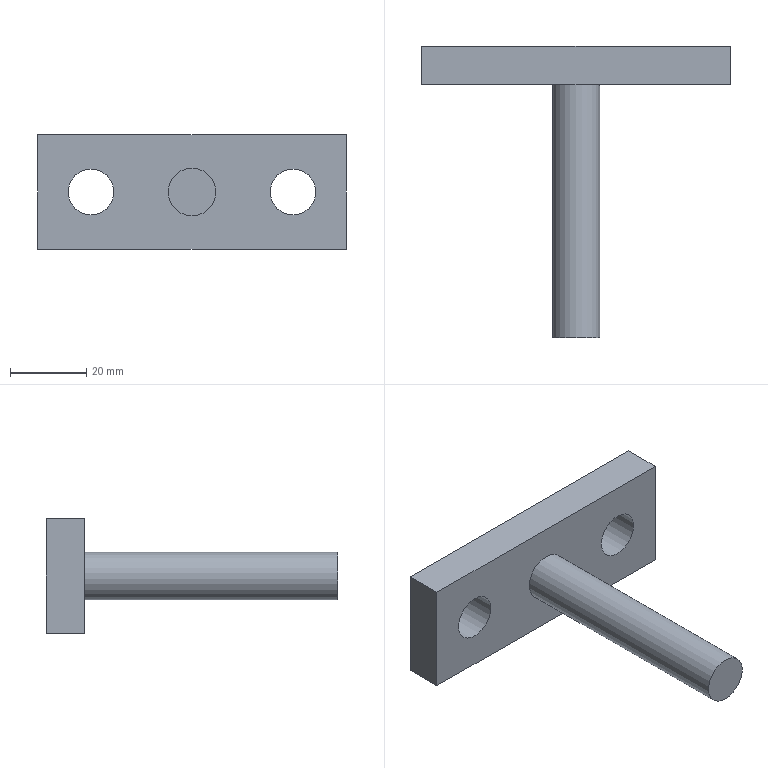Part | STEP file | Tube necking machine_id10_x_t | 1 solid | 10 faces | box 81 x 76.5 x 30 mm | volume 30169 mm3 | plane 7 | cylinder 3 | commonest cylinder face diameters 12 x2 12.477 x1
STEP:
#1=CARTESIAN_POINT('',(0.,0.,0.));
#2=DIRECTION('',(0.,0.,1.));
#3=DIRECTION('',(1.,0.,0.));
#4=AXIS2_PLACEMENT_3D('',#1,#2,#3);
#5=CARTESIAN_POINT('',(26.5,-259.,195.));
#6=VERTEX_POINT('',#5);
#7=CARTESIAN_POINT('',(26.5,-259.,183.));
#8=VERTEX_POINT('',#7);
#9=CARTESIAN_POINT('',(26.5,-259.,189.));
#10=DIRECTION('',(0.,1.,0.));
#11=DIRECTION('',(0.,0.,-1.));
#12=AXIS2_PLACEMENT_3D('',#9,#10,#11);
#13=CIRCLE('',#12,6.);
#14=CARTESIAN_POINT('',(26.5,-807.,189.));
#15=DIRECTION('',(0.,1.,0.));
#16=DIRECTION('',(0.,0.,1.));
#17=AXIS2_PLACEMENT_3D('',#14,#15,#16);
#18=CYLINDRICAL_SURFACE('',#17,6.);
#19=CARTESIAN_POINT('',(-3.142,548.));
#20=DIRECTION('',(1.,0.));
#21=VECTOR('',#20,1.);
#22=LINE('',#19,#21);
#23=(GEOMETRIC_REPRESENTATION_CONTEXT(2)PARAMETRIC_REPRESENTATION_CONTEXT()REPRESENTATION_CONTEXT('',''));
#24=DEFINITIONAL_REPRESENTATION('',(#22),#23);
#25=PCURVE('',#18,#24);
#26=CARTESIAN_POINT('',(0.,-259.,0.));
#27=DIRECTION('',(0.,-1.,0.));
#28=DIRECTION('',(0.,0.,-1.));
#29=AXIS2_PLACEMENT_3D('',#26,#27,#28);
#30=PLANE('',#29);
#31=CARTESIAN_POINT('',(-183.,26.5));
#32=CARTESIAN_POINT('',(-183.,16.108));
#33=CARTESIAN_POINT('',(-192.,21.304));
#34=CARTESIAN_POINT('',(-201.,26.5));
#35=CARTESIAN_POINT('',(-192.,31.696));
#36=CARTESIAN_POINT('',(-183.,36.892));
#37=CARTESIAN_POINT('',(-183.,26.5));
#38=(BOUNDED_CURVE()B_SPLINE_CURVE(2,(#31,#32,#33,#34,#35,#36,#37),.UNSPECIFIED.,.T.,.F.)B_SPLINE_CURVE_WITH_KNOTS((1,2,2,2,2,1),(-2.094,0.,2.094,4.189,6.283,8.378),.UNSPECIFIED.)CURVE()GEOMETRIC_REPRESENTATION_ITEM()RATIONAL_B_SPLINE_CURVE((1.,0.5,1.,0.5,1.,0.5,1.))REPRESENTATION_ITEM(''));
#39=(GEOMETRIC_REPRESENTATION_CONTEXT(2)PARAMETRIC_REPRESENTATION_CONTEXT()REPRESENTATION_CONTEXT('',''));
#40=DEFINITIONAL_REPRESENTATION('',(#38),#39);
#41=PCURVE('',#30,#40);
#42=SURFACE_CURVE('',#13,(#25,#41),.PCURVE_S1.);
#43=EDGE_CURVE('',#6,#8,#42,.T.);
#44=ORIENTED_EDGE('',*,*,#43,.F.);
#45=CARTESIAN_POINT('',(26.5,-269.,195.));
#46=VERTEX_POINT('',#45);
#47=CARTESIAN_POINT('',(26.5,-269.,195.));
#48=CARTESIAN_POINT('',(26.5,-259.,195.));
#49=B_SPLINE_CURVE_WITH_KNOTS('',1,(#47,#48),.UNSPECIFIED.,.F.,.F.,(2,2),(538.,548.),.PIECEWISE_BEZIER_KNOTS.);
#50=CARTESIAN_POINT('',(0.,0.));
#51=DIRECTION('',(0.,1.));
#52=VECTOR('',#51,1.);
#53=LINE('',#50,#52);
#54=(GEOMETRIC_REPRESENTATION_CONTEXT(2)PARAMETRIC_REPRESENTATION_CONTEXT()REPRESENTATION_CONTEXT('',''));
#55=DEFINITIONAL_REPRESENTATION('',(#53),#54);
#56=PCURVE('',#18,#55);
#57=CARTESIAN_POINT('',(6.283,0.));
#58=DIRECTION('',(0.,1.));
#59=VECTOR('',#58,1.);
#60=LINE('',#57,#59);
#61=(GEOMETRIC_REPRESENTATION_CONTEXT(2)PARAMETRIC_REPRESENTATION_CONTEXT()REPRESENTATION_CONTEXT('',''));
#62=DEFINITIONAL_REPRESENTATION('',(#60),#61);
#63=PCURVE('',#18,#62);
#64=SEAM_CURVE('',#49,(#56,#63),.PCURVE_S1.);
#65=EDGE_CURVE('',#46,#6,#64,.T.);
#66=ORIENTED_EDGE('',*,*,#65,.F.);
#67=CARTESIAN_POINT('',(26.5,-269.,189.));
#68=DIRECTION('',(0.,-1.,0.));
#69=DIRECTION('',(0.,0.,1.));
#70=AXIS2_PLACEMENT_3D('',#67,#68,#69);
#71=CIRCLE('',#70,6.);
#72=CARTESIAN_POINT('',(6.283,538.));
#73=DIRECTION('',(-1.,0.));
#74=VECTOR('',#73,1.);
#75=LINE('',#72,#74);
#76=(GEOMETRIC_REPRESENTATION_CONTEXT(2)PARAMETRIC_REPRESENTATION_CONTEXT()REPRESENTATION_CONTEXT('',''));
#77=DEFINITIONAL_REPRESENTATION('',(#75),#76);
#78=PCURVE('',#18,#77);
#79=CARTESIAN_POINT('',(0.,-269.,0.));
#80=DIRECTION('',(0.,1.,0.));
#81=DIRECTION('',(0.,0.,1.));
#82=AXIS2_PLACEMENT_3D('',#79,#80,#81);
#83=PLANE('',#82);
#84=CARTESIAN_POINT('',(195.,26.5));
#85=CARTESIAN_POINT('',(195.,16.108));
#86=CARTESIAN_POINT('',(186.,21.304));
#87=CARTESIAN_POINT('',(177.,26.5));
#88=CARTESIAN_POINT('',(186.,31.696));
#89=CARTESIAN_POINT('',(195.,36.892));
#90=CARTESIAN_POINT('',(195.,26.5));
#91=(BOUNDED_CURVE()B_SPLINE_CURVE(2,(#84,#85,#86,#87,#88,#89,#90),.UNSPECIFIED.,.T.,.F.)B_SPLINE_CURVE_WITH_KNOTS((1,2,2,2,2,1),(-2.094,0.,2.094,4.189,6.283,8.378),.UNSPECIFIED.)CURVE()GEOMETRIC_REPRESENTATION_ITEM()RATIONAL_B_SPLINE_CURVE((1.,0.5,1.,0.5,1.,0.5,1.))REPRESENTATION_ITEM(''));
#92=(GEOMETRIC_REPRESENTATION_CONTEXT(2)PARAMETRIC_REPRESENTATION_CONTEXT()REPRESENTATION_CONTEXT('',''));
#93=DEFINITIONAL_REPRESENTATION('',(#91),#92);
#94=PCURVE('',#83,#93);
#95=SURFACE_CURVE('',#71,(#78,#94),.PCURVE_S1.);
#96=EDGE_CURVE('',#46,#46,#95,.T.);
#97=ORIENTED_EDGE('',*,*,#96,.F.);
#98=ORIENTED_EDGE('',*,*,#65,.T.);
#99=CARTESIAN_POINT('',(26.5,-259.,189.));
#100=DIRECTION('',(0.,1.,0.));
#101=DIRECTION('',(0.,0.,-1.));
#102=AXIS2_PLACEMENT_3D('',#99,#100,#101);
#103=CIRCLE('',#102,6.);
#104=CARTESIAN_POINT('',(3.142,548.));
#105=DIRECTION('',(1.,0.));
#106=VECTOR('',#105,1.);
#107=LINE('',#104,#106);
#108=(GEOMETRIC_REPRESENTATION_CONTEXT(2)PARAMETRIC_REPRESENTATION_CONTEXT()REPRESENTATION_CONTEXT('',''));
#109=DEFINITIONAL_REPRESENTATION('',(#107),#108);
#110=PCURVE('',#18,#109);
#111=CARTESIAN_POINT('',(-183.,26.5));
#112=CARTESIAN_POINT('',(-183.,16.108));
#113=CARTESIAN_POINT('',(-192.,21.304));
#114=CARTESIAN_POINT('',(-201.,26.5));
#115=CARTESIAN_POINT('',(-192.,31.696));
#116=CARTESIAN_POINT('',(-183.,36.892));
#117=CARTESIAN_POINT('',(-183.,26.5));
#118=(BOUNDED_CURVE()B_SPLINE_CURVE(2,(#111,#112,#113,#114,#115,#116,#117),.UNSPECIFIED.,.T.,.F.)B_SPLINE_CURVE_WITH_KNOTS((1,2,2,2,2,1),(-2.094,0.,2.094,4.189,6.283,8.378),.UNSPECIFIED.)CURVE()GEOMETRIC_REPRESENTATION_ITEM()RATIONAL_B_SPLINE_CURVE((1.,0.5,1.,0.5,1.,0.5,1.))REPRESENTATION_ITEM(''));
#119=(GEOMETRIC_REPRESENTATION_CONTEXT(2)PARAMETRIC_REPRESENTATION_CONTEXT()REPRESENTATION_CONTEXT('',''));
#120=DEFINITIONAL_REPRESENTATION('',(#118),#119);
#121=PCURVE('',#30,#120);
#122=SURFACE_CURVE('',#103,(#110,#121),.PCURVE_S1.);
#123=EDGE_CURVE('',#8,#6,#122,.T.);
#124=ORIENTED_EDGE('',*,*,#123,.F.);
#125=EDGE_LOOP('',(#44,#66,#97,#98,#124));
#126=FACE_BOUND('',#125,.F.);
#127=ADVANCED_FACE('',(#126),#18,.F.);
#128=CARTESIAN_POINT('',(0.,-335.5,182.761));
#129=VERTEX_POINT('',#128);
#130=CARTESIAN_POINT('',(0.,-335.5,189.));
#131=DIRECTION('',(0.,1.,0.));
#132=DIRECTION('',(0.,0.,-1.));
#133=AXIS2_PLACEMENT_3D('',#130,#131,#132);
#134=CIRCLE('',#133,6.239);
#135=CARTESIAN_POINT('',(-26.5,-335.5,189.));
#136=DIRECTION('',(0.,-1.,0.));
#137=DIRECTION('',(0.,0.,-1.));
#138=AXIS2_PLACEMENT_3D('',#135,#136,#137);
#139=PLANE('',#138);
#140=CARTESIAN_POINT('',(6.239,26.5));
#141=CARTESIAN_POINT('',(6.239,15.694));
#142=CARTESIAN_POINT('',(-3.119,21.097));
#143=CARTESIAN_POINT('',(-12.477,26.5));
#144=CARTESIAN_POINT('',(-3.119,31.903));
#145=CARTESIAN_POINT('',(6.239,37.306));
#146=CARTESIAN_POINT('',(6.239,26.5));
#147=(BOUNDED_CURVE()B_SPLINE_CURVE(2,(#140,#141,#142,#143,#144,#145,#146),.UNSPECIFIED.,.T.,.F.)B_SPLINE_CURVE_WITH_KNOTS((1,2,2,2,2,1),(-2.094,0.,2.094,4.189,6.283,8.378),.UNSPECIFIED.)CURVE()GEOMETRIC_REPRESENTATION_ITEM()RATIONAL_B_SPLINE_CURVE((1.,0.5,1.,0.5,1.,0.5,1.))REPRESENTATION_ITEM(''));
#148=(GEOMETRIC_REPRESENTATION_CONTEXT(2)PARAMETRIC_REPRESENTATION_CONTEXT()REPRESENTATION_CONTEXT('',''));
#149=DEFINITIONAL_REPRESENTATION('',(#147),#148);
#150=PCURVE('',#139,#149);
#151=CARTESIAN_POINT('',(0.,-262.,189.));
#152=DIRECTION('',(0.,-1.,0.));
#153=DIRECTION('',(0.,0.,-1.));
#154=AXIS2_PLACEMENT_3D('',#151,#152,#153);
#155=CYLINDRICAL_SURFACE('',#154,6.239);
#156=CARTESIAN_POINT('',(6.283,73.5));
#157=DIRECTION('',(-1.,0.));
#158=VECTOR('',#157,1.);
#159=LINE('',#156,#158);
#160=(GEOMETRIC_REPRESENTATION_CONTEXT(2)PARAMETRIC_REPRESENTATION_CONTEXT()REPRESENTATION_CONTEXT('',''));
#161=DEFINITIONAL_REPRESENTATION('',(#159),#160);
#162=PCURVE('',#155,#161);
#163=SURFACE_CURVE('',#134,(#150,#162),.PCURVE_S1.);
#164=EDGE_CURVE('',#129,#129,#163,.T.);
#165=ORIENTED_EDGE('',*,*,#164,.F.);
#166=EDGE_LOOP('',(#165));
#167=FACE_BOUND('',#166,.T.);
#168=ADVANCED_FACE('',(#167),#139,.T.);
#169=ORIENTED_EDGE('',*,*,#164,.T.);
#170=CARTESIAN_POINT('',(0.,-269.,182.761));
#171=VERTEX_POINT('',#170);
#172=CARTESIAN_POINT('',(0.,-269.,182.761));
#173=CARTESIAN_POINT('',(0.,-335.5,182.761));
#174=B_SPLINE_CURVE_WITH_KNOTS('',1,(#172,#173),.UNSPECIFIED.,.F.,.F.,(2,2),(7.,73.5),.PIECEWISE_BEZIER_KNOTS.);
#175=CARTESIAN_POINT('',(0.,0.));
#176=DIRECTION('',(0.,1.));
#177=VECTOR('',#176,1.);
#178=LINE('',#175,#177);
#179=(GEOMETRIC_REPRESENTATION_CONTEXT(2)PARAMETRIC_REPRESENTATION_CONTEXT()REPRESENTATION_CONTEXT('',''));
#180=DEFINITIONAL_REPRESENTATION('',(#178),#179);
#181=PCURVE('',#155,#180);
#182=CARTESIAN_POINT('',(6.283,0.));
#183=DIRECTION('',(0.,1.));
#184=VECTOR('',#183,1.);
#185=LINE('',#182,#184);
#186=(GEOMETRIC_REPRESENTATION_CONTEXT(2)PARAMETRIC_REPRESENTATION_CONTEXT()REPRESENTATION_CONTEXT('',''));
#187=DEFINITIONAL_REPRESENTATION('',(#185),#186);
#188=PCURVE('',#155,#187);
#189=SEAM_CURVE('',#174,(#181,#188),.PCURVE_S1.);
#190=EDGE_CURVE('',#171,#129,#189,.T.);
#191=ORIENTED_EDGE('',*,*,#190,.F.);
#192=CARTESIAN_POINT('',(0.,-269.,195.239));
#193=VERTEX_POINT('',#192);
#194=CARTESIAN_POINT('',(0.,-269.,189.));
#195=DIRECTION('',(0.,1.,0.));
#196=DIRECTION('',(0.,0.,1.));
#197=AXIS2_PLACEMENT_3D('',#194,#195,#196);
#198=CIRCLE('',#197,6.239);
#199=CARTESIAN_POINT('',(3.142,7.));
#200=DIRECTION('',(-1.,0.));
#201=VECTOR('',#200,1.);
#202=LINE('',#199,#201);
#203=(GEOMETRIC_REPRESENTATION_CONTEXT(2)PARAMETRIC_REPRESENTATION_CONTEXT()REPRESENTATION_CONTEXT('',''));
#204=DEFINITIONAL_REPRESENTATION('',(#202),#203);
#205=PCURVE('',#155,#204);
#206=CARTESIAN_POINT('',(189.,0.));
#207=DIRECTION('',(1.,0.));
#208=AXIS2_PLACEMENT_2D('',#206,#207);
#209=CIRCLE('',#208,6.239);
#210=(GEOMETRIC_REPRESENTATION_CONTEXT(2)PARAMETRIC_REPRESENTATION_CONTEXT()REPRESENTATION_CONTEXT('',''));
#211=DEFINITIONAL_REPRESENTATION('',(#209),#210);
#212=PCURVE('',#83,#211);
#213=SURFACE_CURVE('',#198,(#205,#212),.PCURVE_S1.);
#214=EDGE_CURVE('',#193,#171,#213,.T.);
#215=ORIENTED_EDGE('',*,*,#214,.F.);
#216=CARTESIAN_POINT('',(0.,-269.,189.));
#217=DIRECTION('',(0.,1.,0.));
#218=DIRECTION('',(0.,0.,1.));
#219=AXIS2_PLACEMENT_3D('',#216,#217,#218);
#220=CIRCLE('',#219,6.239);
#221=CARTESIAN_POINT('',(9.425,7.));
#222=DIRECTION('',(-1.,0.));
#223=VECTOR('',#222,1.);
#224=LINE('',#221,#223);
#225=(GEOMETRIC_REPRESENTATION_CONTEXT(2)PARAMETRIC_REPRESENTATION_CONTEXT()REPRESENTATION_CONTEXT('',''));
#226=DEFINITIONAL_REPRESENTATION('',(#224),#225);
#227=PCURVE('',#155,#226);
#228=CARTESIAN_POINT('',(189.,0.));
#229=DIRECTION('',(1.,0.));
#230=AXIS2_PLACEMENT_2D('',#228,#229);
#231=CIRCLE('',#230,6.239);
#232=(GEOMETRIC_REPRESENTATION_CONTEXT(2)PARAMETRIC_REPRESENTATION_CONTEXT()REPRESENTATION_CONTEXT('',''));
#233=DEFINITIONAL_REPRESENTATION('',(#231),#232);
#234=PCURVE('',#83,#233);
#235=SURFACE_CURVE('',#220,(#227,#234),.PCURVE_S1.);
#236=EDGE_CURVE('',#171,#193,#235,.T.);
#237=ORIENTED_EDGE('',*,*,#236,.F.);
#238=ORIENTED_EDGE('',*,*,#190,.T.);
#239=EDGE_LOOP('',(#169,#191,#215,#237,#238));
#240=FACE_BOUND('',#239,.T.);
#241=ADVANCED_FACE('',(#240),#155,.T.);
#242=CARTESIAN_POINT('',(-40.5,-259.,204.));
#243=VERTEX_POINT('',#242);
#244=CARTESIAN_POINT('',(-40.5,-269.,204.));
#245=VERTEX_POINT('',#244);
#246=CARTESIAN_POINT('',(-40.5,-125.5,204.));
#247=DIRECTION('',(0.,-1.,0.));
#248=VECTOR('',#247,1.);
#249=LINE('',#246,#248);
#250=CARTESIAN_POINT('',(-40.5,-125.5,171.));
#251=DIRECTION('',(1.,0.,0.));
#252=DIRECTION('',(0.,0.,-1.));
#253=AXIS2_PLACEMENT_3D('',#250,#251,#252);
#254=PLANE('',#253);
#255=CARTESIAN_POINT('',(-33.,0.));
#256=DIRECTION('',(0.,-1.));
#257=VECTOR('',#256,1.);
#258=LINE('',#255,#257);
#259=(GEOMETRIC_REPRESENTATION_CONTEXT(2)PARAMETRIC_REPRESENTATION_CONTEXT()REPRESENTATION_CONTEXT('',''));
#260=DEFINITIONAL_REPRESENTATION('',(#258),#259);
#261=PCURVE('',#254,#260);
#262=CARTESIAN_POINT('',(-41.5,-125.5,204.));
#263=DIRECTION('',(0.,0.,-1.));
#264=DIRECTION('',(-1.,0.,0.));
#265=AXIS2_PLACEMENT_3D('',#262,#263,#264);
#266=PLANE('',#265);
#267=CARTESIAN_POINT('',(-1.,0.));
#268=DIRECTION('',(0.,-1.));
#269=VECTOR('',#268,1.);
#270=LINE('',#267,#269);
#271=(GEOMETRIC_REPRESENTATION_CONTEXT(2)PARAMETRIC_REPRESENTATION_CONTEXT()REPRESENTATION_CONTEXT('',''));
#272=DEFINITIONAL_REPRESENTATION('',(#270),#271);
#273=PCURVE('',#266,#272);
#274=SURFACE_CURVE('',#249,(#261,#273),.PCURVE_S1.);
#275=EDGE_CURVE('',#243,#245,#274,.T.);
#276=ORIENTED_EDGE('',*,*,#275,.F.);
#277=CARTESIAN_POINT('',(-40.5,-259.,174.));
#278=VERTEX_POINT('',#277);
#279=CARTESIAN_POINT('',(-40.5,-259.,171.));
#280=DIRECTION('',(0.,0.,-1.));
#281=VECTOR('',#280,1.);
#282=LINE('',#279,#281);
#283=CARTESIAN_POINT('',(0.,-133.5));
#284=DIRECTION('',(1.,0.));
#285=VECTOR('',#284,1.);
#286=LINE('',#283,#285);
#287=(GEOMETRIC_REPRESENTATION_CONTEXT(2)PARAMETRIC_REPRESENTATION_CONTEXT()REPRESENTATION_CONTEXT('',''));
#288=DEFINITIONAL_REPRESENTATION('',(#286),#287);
#289=PCURVE('',#254,#288);
#290=CARTESIAN_POINT('',(-171.,-40.5));
#291=DIRECTION('',(1.,0.));
#292=VECTOR('',#291,1.);
#293=LINE('',#290,#292);
#294=(GEOMETRIC_REPRESENTATION_CONTEXT(2)PARAMETRIC_REPRESENTATION_CONTEXT()REPRESENTATION_CONTEXT('',''));
#295=DEFINITIONAL_REPRESENTATION('',(#293),#294);
#296=PCURVE('',#30,#295);
#297=SURFACE_CURVE('',#282,(#289,#296),.PCURVE_S1.);
#298=EDGE_CURVE('',#243,#278,#297,.T.);
#299=ORIENTED_EDGE('',*,*,#298,.T.);
#300=CARTESIAN_POINT('',(-40.5,-269.,174.));
#301=VERTEX_POINT('',#300);
#302=CARTESIAN_POINT('',(-40.5,-125.5,174.));
#303=DIRECTION('',(0.,-1.,0.));
#304=VECTOR('',#303,1.);
#305=LINE('',#302,#304);
#306=CARTESIAN_POINT('',(-3.,0.));
#307=DIRECTION('',(0.,-1.));
#308=VECTOR('',#307,1.);
#309=LINE('',#306,#308);
#310=(GEOMETRIC_REPRESENTATION_CONTEXT(2)PARAMETRIC_REPRESENTATION_CONTEXT()REPRESENTATION_CONTEXT('',''));
#311=DEFINITIONAL_REPRESENTATION('',(#309),#310);
#312=PCURVE('',#254,#311);
#313=CARTESIAN_POINT('',(41.5,-125.5,174.));
#314=DIRECTION('',(0.,0.,1.));
#315=DIRECTION('',(1.,0.,0.));
#316=AXIS2_PLACEMENT_3D('',#313,#314,#315);
#317=PLANE('',#316);
#318=CARTESIAN_POINT('',(-82.,0.));
#319=DIRECTION('',(0.,-1.));
#320=VECTOR('',#319,1.);
#321=LINE('',#318,#320);
#322=(GEOMETRIC_REPRESENTATION_CONTEXT(2)PARAMETRIC_REPRESENTATION_CONTEXT()REPRESENTATION_CONTEXT('',''));
#323=DEFINITIONAL_REPRESENTATION('',(#321),#322);
#324=PCURVE('',#317,#323);
#325=SURFACE_CURVE('',#305,(#312,#324),.PCURVE_S1.);
#326=EDGE_CURVE('',#278,#301,#325,.T.);
#327=ORIENTED_EDGE('',*,*,#326,.T.);
#328=CARTESIAN_POINT('',(-40.5,-269.,171.));
#329=DIRECTION('',(0.,0.,1.));
#330=VECTOR('',#329,1.);
#331=LINE('',#328,#330);
#332=CARTESIAN_POINT('',(0.,-143.5));
#333=DIRECTION('',(-1.,0.));
#334=VECTOR('',#333,1.);
#335=LINE('',#332,#334);
#336=(GEOMETRIC_REPRESENTATION_CONTEXT(2)PARAMETRIC_REPRESENTATION_CONTEXT()REPRESENTATION_CONTEXT('',''));
#337=DEFINITIONAL_REPRESENTATION('',(#335),#336);
#338=PCURVE('',#254,#337);
#339=CARTESIAN_POINT('',(171.,-40.5));
#340=DIRECTION('',(1.,0.));
#341=VECTOR('',#340,1.);
#342=LINE('',#339,#341);
#343=(GEOMETRIC_REPRESENTATION_CONTEXT(2)PARAMETRIC_REPRESENTATION_CONTEXT()REPRESENTATION_CONTEXT('',''));
#344=DEFINITIONAL_REPRESENTATION('',(#342),#343);
#345=PCURVE('',#83,#344);
#346=SURFACE_CURVE('',#331,(#338,#345),.PCURVE_S1.);
#347=EDGE_CURVE('',#301,#245,#346,.T.);
#348=ORIENTED_EDGE('',*,*,#347,.T.);
#349=EDGE_LOOP('',(#276,#299,#327,#348));
#350=FACE_BOUND('',#349,.T.);
#351=ADVANCED_FACE('',(#350),#254,.F.);
#352=ORIENTED_EDGE('',*,*,#326,.F.);
#353=CARTESIAN_POINT('',(40.5,-259.,174.));
#354=VERTEX_POINT('',#353);
#355=CARTESIAN_POINT('',(41.5,-259.,174.));
#356=DIRECTION('',(1.,0.,0.));
#357=VECTOR('',#356,1.);
#358=LINE('',#355,#357);
#359=CARTESIAN_POINT('',(0.,-133.5));
#360=DIRECTION('',(1.,0.));
#361=VECTOR('',#360,1.);
#362=LINE('',#359,#361);
#363=(GEOMETRIC_REPRESENTATION_CONTEXT(2)PARAMETRIC_REPRESENTATION_CONTEXT()REPRESENTATION_CONTEXT('',''));
#364=DEFINITIONAL_REPRESENTATION('',(#362),#363);
#365=PCURVE('',#317,#364);
#366=CARTESIAN_POINT('',(-174.,41.5));
#367=DIRECTION('',(0.,1.));
#368=VECTOR('',#367,1.);
#369=LINE('',#366,#368);
#370=(GEOMETRIC_REPRESENTATION_CONTEXT(2)PARAMETRIC_REPRESENTATION_CONTEXT()REPRESENTATION_CONTEXT('',''));
#371=DEFINITIONAL_REPRESENTATION('',(#369),#370);
#372=PCURVE('',#30,#371);
#373=SURFACE_CURVE('',#358,(#365,#372),.PCURVE_S1.);
#374=EDGE_CURVE('',#278,#354,#373,.T.);
#375=ORIENTED_EDGE('',*,*,#374,.T.);
#376=CARTESIAN_POINT('',(40.5,-269.,174.));
#377=VERTEX_POINT('',#376);
#378=CARTESIAN_POINT('',(40.5,-125.5,174.));
#379=DIRECTION('',(0.,-1.,0.));
#380=VECTOR('',#379,1.);
#381=LINE('',#378,#380);
#382=CARTESIAN_POINT('',(-1.,0.));
#383=DIRECTION('',(0.,-1.));
#384=VECTOR('',#383,1.);
#385=LINE('',#382,#384);
#386=(GEOMETRIC_REPRESENTATION_CONTEXT(2)PARAMETRIC_REPRESENTATION_CONTEXT()REPRESENTATION_CONTEXT('',''));
#387=DEFINITIONAL_REPRESENTATION('',(#385),#386);
#388=PCURVE('',#317,#387);
#389=CARTESIAN_POINT('',(40.5,-125.5,207.));
#390=DIRECTION('',(-1.,0.,0.));
#391=DIRECTION('',(0.,0.,1.));
#392=AXIS2_PLACEMENT_3D('',#389,#390,#391);
#393=PLANE('',#392);
#394=CARTESIAN_POINT('',(-33.,0.));
#395=DIRECTION('',(0.,-1.));
#396=VECTOR('',#395,1.);
#397=LINE('',#394,#396);
#398=(GEOMETRIC_REPRESENTATION_CONTEXT(2)PARAMETRIC_REPRESENTATION_CONTEXT()REPRESENTATION_CONTEXT('',''));
#399=DEFINITIONAL_REPRESENTATION('',(#397),#398);
#400=PCURVE('',#393,#399);
#401=SURFACE_CURVE('',#381,(#388,#400),.PCURVE_S1.);
#402=EDGE_CURVE('',#354,#377,#401,.T.);
#403=ORIENTED_EDGE('',*,*,#402,.T.);
#404=CARTESIAN_POINT('',(41.5,-269.,174.));
#405=DIRECTION('',(-1.,0.,0.));
#406=VECTOR('',#405,1.);
#407=LINE('',#404,#406);
#408=CARTESIAN_POINT('',(0.,-143.5));
#409=DIRECTION('',(-1.,0.));
#410=VECTOR('',#409,1.);
#411=LINE('',#408,#410);
#412=(GEOMETRIC_REPRESENTATION_CONTEXT(2)PARAMETRIC_REPRESENTATION_CONTEXT()REPRESENTATION_CONTEXT('',''));
#413=DEFINITIONAL_REPRESENTATION('',(#411),#412);
#414=PCURVE('',#317,#413);
#415=CARTESIAN_POINT('',(174.,41.5));
#416=DIRECTION('',(0.,-1.));
#417=VECTOR('',#416,1.);
#418=LINE('',#415,#417);
#419=(GEOMETRIC_REPRESENTATION_CONTEXT(2)PARAMETRIC_REPRESENTATION_CONTEXT()REPRESENTATION_CONTEXT('',''));
#420=DEFINITIONAL_REPRESENTATION('',(#418),#419);
#421=PCURVE('',#83,#420);
#422=SURFACE_CURVE('',#407,(#414,#421),.PCURVE_S1.);
#423=EDGE_CURVE('',#377,#301,#422,.T.);
#424=ORIENTED_EDGE('',*,*,#423,.T.);
#425=EDGE_LOOP('',(#352,#375,#403,#424));
#426=FACE_BOUND('',#425,.T.);
#427=ADVANCED_FACE('',(#426),#317,.F.);
#428=ORIENTED_EDGE('',*,*,#402,.F.);
#429=CARTESIAN_POINT('',(40.5,-259.,204.));
#430=VERTEX_POINT('',#429);
#431=CARTESIAN_POINT('',(40.5,-259.,207.));
#432=DIRECTION('',(0.,0.,1.));
#433=VECTOR('',#432,1.);
#434=LINE('',#431,#433);
#435=CARTESIAN_POINT('',(0.,-133.5));
#436=DIRECTION('',(1.,0.));
#437=VECTOR('',#436,1.);
#438=LINE('',#435,#437);
#439=(GEOMETRIC_REPRESENTATION_CONTEXT(2)PARAMETRIC_REPRESENTATION_CONTEXT()REPRESENTATION_CONTEXT('',''));
#440=DEFINITIONAL_REPRESENTATION('',(#438),#439);
#441=PCURVE('',#393,#440);
#442=CARTESIAN_POINT('',(-207.,40.5));
#443=DIRECTION('',(-1.,0.));
#444=VECTOR('',#443,1.);
#445=LINE('',#442,#444);
#446=(GEOMETRIC_REPRESENTATION_CONTEXT(2)PARAMETRIC_REPRESENTATION_CONTEXT()REPRESENTATION_CONTEXT('',''));
#447=DEFINITIONAL_REPRESENTATION('',(#445),#446);
#448=PCURVE('',#30,#447);
#449=SURFACE_CURVE('',#434,(#441,#448),.PCURVE_S1.);
#450=EDGE_CURVE('',#354,#430,#449,.T.);
#451=ORIENTED_EDGE('',*,*,#450,.T.);
#452=CARTESIAN_POINT('',(40.5,-269.,204.));
#453=VERTEX_POINT('',#452);
#454=CARTESIAN_POINT('',(40.5,-125.5,204.));
#455=DIRECTION('',(0.,-1.,0.));
#456=VECTOR('',#455,1.);
#457=LINE('',#454,#456);
#458=CARTESIAN_POINT('',(-3.,0.));
#459=DIRECTION('',(0.,-1.));
#460=VECTOR('',#459,1.);
#461=LINE('',#458,#460);
#462=(GEOMETRIC_REPRESENTATION_CONTEXT(2)PARAMETRIC_REPRESENTATION_CONTEXT()REPRESENTATION_CONTEXT('',''));
#463=DEFINITIONAL_REPRESENTATION('',(#461),#462);
#464=PCURVE('',#393,#463);
#465=CARTESIAN_POINT('',(-82.,0.));
#466=DIRECTION('',(0.,-1.));
#467=VECTOR('',#466,1.);
#468=LINE('',#465,#467);
#469=(GEOMETRIC_REPRESENTATION_CONTEXT(2)PARAMETRIC_REPRESENTATION_CONTEXT()REPRESENTATION_CONTEXT('',''));
#470=DEFINITIONAL_REPRESENTATION('',(#468),#469);
#471=PCURVE('',#266,#470);
#472=SURFACE_CURVE('',#457,(#464,#471),.PCURVE_S1.);
#473=EDGE_CURVE('',#430,#453,#472,.T.);
#474=ORIENTED_EDGE('',*,*,#473,.T.);
#475=CARTESIAN_POINT('',(40.5,-269.,207.));
#476=DIRECTION('',(0.,0.,-1.));
#477=VECTOR('',#476,1.);
#478=LINE('',#475,#477);
#479=CARTESIAN_POINT('',(0.,-143.5));
#480=DIRECTION('',(-1.,0.));
#481=VECTOR('',#480,1.);
#482=LINE('',#479,#481);
#483=(GEOMETRIC_REPRESENTATION_CONTEXT(2)PARAMETRIC_REPRESENTATION_CONTEXT()REPRESENTATION_CONTEXT('',''));
#484=DEFINITIONAL_REPRESENTATION('',(#482),#483);
#485=PCURVE('',#393,#484);
#486=CARTESIAN_POINT('',(207.,40.5));
#487=DIRECTION('',(-1.,0.));
#488=VECTOR('',#487,1.);
#489=LINE('',#486,#488);
#490=(GEOMETRIC_REPRESENTATION_CONTEXT(2)PARAMETRIC_REPRESENTATION_CONTEXT()REPRESENTATION_CONTEXT('',''));
#491=DEFINITIONAL_REPRESENTATION('',(#489),#490);
#492=PCURVE('',#83,#491);
#493=SURFACE_CURVE('',#478,(#485,#492),.PCURVE_S1.);
#494=EDGE_CURVE('',#453,#377,#493,.T.);
#495=ORIENTED_EDGE('',*,*,#494,.T.);
#496=EDGE_LOOP('',(#428,#451,#474,#495));
#497=FACE_BOUND('',#496,.T.);
#498=ADVANCED_FACE('',(#497),#393,.F.);
#499=ORIENTED_EDGE('',*,*,#473,.F.);
#500=CARTESIAN_POINT('',(-41.5,-259.,204.));
#501=DIRECTION('',(-1.,0.,0.));
#502=VECTOR('',#501,1.);
#503=LINE('',#500,#502);
#504=CARTESIAN_POINT('',(0.,-133.5));
#505=DIRECTION('',(1.,0.));
#506=VECTOR('',#505,1.);
#507=LINE('',#504,#506);
#508=(GEOMETRIC_REPRESENTATION_CONTEXT(2)PARAMETRIC_REPRESENTATION_CONTEXT()REPRESENTATION_CONTEXT('',''));
#509=DEFINITIONAL_REPRESENTATION('',(#507),#508);
#510=PCURVE('',#266,#509);
#511=CARTESIAN_POINT('',(-204.,-41.5));
#512=DIRECTION('',(0.,-1.));
#513=VECTOR('',#512,1.);
#514=LINE('',#511,#513);
#515=(GEOMETRIC_REPRESENTATION_CONTEXT(2)PARAMETRIC_REPRESENTATION_CONTEXT()REPRESENTATION_CONTEXT('',''));
#516=DEFINITIONAL_REPRESENTATION('',(#514),#515);
#517=PCURVE('',#30,#516);
#518=SURFACE_CURVE('',#503,(#510,#517),.PCURVE_S1.);
#519=EDGE_CURVE('',#430,#243,#518,.T.);
#520=ORIENTED_EDGE('',*,*,#519,.T.);
#521=ORIENTED_EDGE('',*,*,#275,.T.);
#522=CARTESIAN_POINT('',(-41.5,-269.,204.));
#523=DIRECTION('',(1.,0.,0.));
#524=VECTOR('',#523,1.);
#525=LINE('',#522,#524);
#526=CARTESIAN_POINT('',(0.,-143.5));
#527=DIRECTION('',(-1.,0.));
#528=VECTOR('',#527,1.);
#529=LINE('',#526,#528);
#530=(GEOMETRIC_REPRESENTATION_CONTEXT(2)PARAMETRIC_REPRESENTATION_CONTEXT()REPRESENTATION_CONTEXT('',''));
#531=DEFINITIONAL_REPRESENTATION('',(#529),#530);
#532=PCURVE('',#266,#531);
#533=CARTESIAN_POINT('',(204.,-41.5));
#534=DIRECTION('',(0.,1.));
#535=VECTOR('',#534,1.);
#536=LINE('',#533,#535);
#537=(GEOMETRIC_REPRESENTATION_CONTEXT(2)PARAMETRIC_REPRESENTATION_CONTEXT()REPRESENTATION_CONTEXT('',''));
#538=DEFINITIONAL_REPRESENTATION('',(#536),#537);
#539=PCURVE('',#83,#538);
#540=SURFACE_CURVE('',#525,(#532,#539),.PCURVE_S1.);
#541=EDGE_CURVE('',#245,#453,#540,.T.);
#542=ORIENTED_EDGE('',*,*,#541,.T.);
#543=EDGE_LOOP('',(#499,#520,#521,#542));
#544=FACE_BOUND('',#543,.T.);
#545=ADVANCED_FACE('',(#544),#266,.F.);
#546=ORIENTED_EDGE('',*,*,#214,.T.);
#547=ORIENTED_EDGE('',*,*,#236,.T.);
#548=EDGE_LOOP('',(#546,#547));
#549=FACE_BOUND('',#548,.T.);
#550=ORIENTED_EDGE('',*,*,#96,.F.);
#551=EDGE_LOOP('',(#550));
#552=FACE_BOUND('',#551,.T.);
#553=CARTESIAN_POINT('',(-26.5,-269.,195.));
#554=VERTEX_POINT('',#553);
#555=CARTESIAN_POINT('',(-26.5,-269.,189.));
#556=DIRECTION('',(0.,1.,0.));
#557=DIRECTION('',(0.,0.,1.));
#558=AXIS2_PLACEMENT_3D('',#555,#556,#557);
#559=CIRCLE('',#558,6.);
#560=CARTESIAN_POINT('',(189.,-26.5));
#561=DIRECTION('',(1.,0.));
#562=AXIS2_PLACEMENT_2D('',#560,#561);
#563=CIRCLE('',#562,6.);
#564=(GEOMETRIC_REPRESENTATION_CONTEXT(2)PARAMETRIC_REPRESENTATION_CONTEXT()REPRESENTATION_CONTEXT('',''));
#565=DEFINITIONAL_REPRESENTATION('',(#563),#564);
#566=PCURVE('',#83,#565);
#567=CARTESIAN_POINT('',(-26.5,-807.,189.));
#568=DIRECTION('',(0.,1.,0.));
#569=DIRECTION('',(0.,0.,1.));
#570=AXIS2_PLACEMENT_3D('',#567,#568,#569);
#571=CYLINDRICAL_SURFACE('',#570,6.);
#572=CARTESIAN_POINT('',(0.,538.));
#573=DIRECTION('',(1.,0.));
#574=VECTOR('',#573,1.);
#575=LINE('',#572,#574);
#576=(GEOMETRIC_REPRESENTATION_CONTEXT(2)PARAMETRIC_REPRESENTATION_CONTEXT()REPRESENTATION_CONTEXT('',''));
#577=DEFINITIONAL_REPRESENTATION('',(#575),#576);
#578=PCURVE('',#571,#577);
#579=SURFACE_CURVE('',#559,(#566,#578),.PCURVE_S1.);
#580=EDGE_CURVE('',#554,#554,#579,.T.);
#581=ORIENTED_EDGE('',*,*,#580,.T.);
#582=EDGE_LOOP('',(#581));
#583=FACE_BOUND('',#582,.T.);
#584=ORIENTED_EDGE('',*,*,#347,.F.);
#585=ORIENTED_EDGE('',*,*,#423,.F.);
#586=ORIENTED_EDGE('',*,*,#494,.F.);
#587=ORIENTED_EDGE('',*,*,#541,.F.);
#588=EDGE_LOOP('',(#584,#585,#586,#587));
#589=FACE_BOUND('',#588,.T.);
#590=ADVANCED_FACE('',(#549,#552,#583,#589),#83,.F.);
#591=ORIENTED_EDGE('',*,*,#580,.T.);
#592=CARTESIAN_POINT('',(-26.5,-259.,195.));
#593=VERTEX_POINT('',#592);
#594=CARTESIAN_POINT('',(-26.5,-269.,195.));
#595=CARTESIAN_POINT('',(-26.5,-259.,195.));
#596=B_SPLINE_CURVE_WITH_KNOTS('',1,(#594,#595),.UNSPECIFIED.,.F.,.F.,(2,2),(538.,548.),.PIECEWISE_BEZIER_KNOTS.);
#597=CARTESIAN_POINT('',(6.283,0.));
#598=DIRECTION('',(0.,1.));
#599=VECTOR('',#598,1.);
#600=LINE('',#597,#599);
#601=(GEOMETRIC_REPRESENTATION_CONTEXT(2)PARAMETRIC_REPRESENTATION_CONTEXT()REPRESENTATION_CONTEXT('',''));
#602=DEFINITIONAL_REPRESENTATION('',(#600),#601);
#603=PCURVE('',#571,#602);
#604=CARTESIAN_POINT('',(0.,0.));
#605=DIRECTION('',(0.,1.));
#606=VECTOR('',#605,1.);
#607=LINE('',#604,#606);
#608=(GEOMETRIC_REPRESENTATION_CONTEXT(2)PARAMETRIC_REPRESENTATION_CONTEXT()REPRESENTATION_CONTEXT('',''));
#609=DEFINITIONAL_REPRESENTATION('',(#607),#608);
#610=PCURVE('',#571,#609);
#611=SEAM_CURVE('',#596,(#603,#610),.PCURVE_S1.);
#612=EDGE_CURVE('',#554,#593,#611,.T.);
#613=ORIENTED_EDGE('',*,*,#612,.T.);
#614=CARTESIAN_POINT('',(-26.5,-259.,183.));
#615=VERTEX_POINT('',#614);
#616=CARTESIAN_POINT('',(-26.5,-259.,189.));
#617=DIRECTION('',(0.,1.,0.));
#618=DIRECTION('',(0.,0.,-1.));
#619=AXIS2_PLACEMENT_3D('',#616,#617,#618);
#620=CIRCLE('',#619,6.);
#621=CARTESIAN_POINT('',(3.142,548.));
#622=DIRECTION('',(1.,0.));
#623=VECTOR('',#622,1.);
#624=LINE('',#621,#623);
#625=(GEOMETRIC_REPRESENTATION_CONTEXT(2)PARAMETRIC_REPRESENTATION_CONTEXT()REPRESENTATION_CONTEXT('',''));
#626=DEFINITIONAL_REPRESENTATION('',(#624),#625);
#627=PCURVE('',#571,#626);
#628=CARTESIAN_POINT('',(-183.,-26.5));
#629=CARTESIAN_POINT('',(-183.,-36.892));
#630=CARTESIAN_POINT('',(-192.,-31.696));
#631=CARTESIAN_POINT('',(-201.,-26.5));
#632=CARTESIAN_POINT('',(-192.,-21.304));
#633=CARTESIAN_POINT('',(-183.,-16.108));
#634=CARTESIAN_POINT('',(-183.,-26.5));
#635=(BOUNDED_CURVE()B_SPLINE_CURVE(2,(#628,#629,#630,#631,#632,#633,#634),.UNSPECIFIED.,.T.,.F.)B_SPLINE_CURVE_WITH_KNOTS((1,2,2,2,2,1),(-2.094,0.,2.094,4.189,6.283,8.378),.UNSPECIFIED.)CURVE()GEOMETRIC_REPRESENTATION_ITEM()RATIONAL_B_SPLINE_CURVE((1.,0.5,1.,0.5,1.,0.5,1.))REPRESENTATION_ITEM(''));
#636=(GEOMETRIC_REPRESENTATION_CONTEXT(2)PARAMETRIC_REPRESENTATION_CONTEXT()REPRESENTATION_CONTEXT('',''));
#637=DEFINITIONAL_REPRESENTATION('',(#635),#636);
#638=PCURVE('',#30,#637);
#639=SURFACE_CURVE('',#620,(#627,#638),.PCURVE_S1.);
#640=EDGE_CURVE('',#615,#593,#639,.T.);
#641=ORIENTED_EDGE('',*,*,#640,.F.);
#642=CARTESIAN_POINT('',(-26.5,-259.,189.));
#643=DIRECTION('',(0.,1.,0.));
#644=DIRECTION('',(0.,0.,-1.));
#645=AXIS2_PLACEMENT_3D('',#642,#643,#644);
#646=CIRCLE('',#645,6.);
#647=CARTESIAN_POINT('',(-3.142,548.));
#648=DIRECTION('',(1.,0.));
#649=VECTOR('',#648,1.);
#650=LINE('',#647,#649);
#651=(GEOMETRIC_REPRESENTATION_CONTEXT(2)PARAMETRIC_REPRESENTATION_CONTEXT()REPRESENTATION_CONTEXT('',''));
#652=DEFINITIONAL_REPRESENTATION('',(#650),#651);
#653=PCURVE('',#571,#652);
#654=CARTESIAN_POINT('',(-183.,-26.5));
#655=CARTESIAN_POINT('',(-183.,-36.892));
#656=CARTESIAN_POINT('',(-192.,-31.696));
#657=CARTESIAN_POINT('',(-201.,-26.5));
#658=CARTESIAN_POINT('',(-192.,-21.304));
#659=CARTESIAN_POINT('',(-183.,-16.108));
#660=CARTESIAN_POINT('',(-183.,-26.5));
#661=(BOUNDED_CURVE()B_SPLINE_CURVE(2,(#654,#655,#656,#657,#658,#659,#660),.UNSPECIFIED.,.T.,.F.)B_SPLINE_CURVE_WITH_KNOTS((1,2,2,2,2,1),(-2.094,0.,2.094,4.189,6.283,8.378),.UNSPECIFIED.)CURVE()GEOMETRIC_REPRESENTATION_ITEM()RATIONAL_B_SPLINE_CURVE((1.,0.5,1.,0.5,1.,0.5,1.))REPRESENTATION_ITEM(''));
#662=(GEOMETRIC_REPRESENTATION_CONTEXT(2)PARAMETRIC_REPRESENTATION_CONTEXT()REPRESENTATION_CONTEXT('',''));
#663=DEFINITIONAL_REPRESENTATION('',(#661),#662);
#664=PCURVE('',#30,#663);
#665=SURFACE_CURVE('',#646,(#653,#664),.PCURVE_S1.);
#666=EDGE_CURVE('',#593,#615,#665,.T.);
#667=ORIENTED_EDGE('',*,*,#666,.F.);
#668=ORIENTED_EDGE('',*,*,#612,.F.);
#669=EDGE_LOOP('',(#591,#613,#641,#667,#668));
#670=FACE_BOUND('',#669,.F.);
#671=ADVANCED_FACE('',(#670),#571,.F.);
#672=ORIENTED_EDGE('',*,*,#123,.F.);
#673=ORIENTED_EDGE('',*,*,#43,.F.);
#674=EDGE_LOOP('',(#672,#673));
#675=FACE_BOUND('',#674,.T.);
#676=ORIENTED_EDGE('',*,*,#640,.F.);
#677=ORIENTED_EDGE('',*,*,#666,.F.);
#678=EDGE_LOOP('',(#676,#677));
#679=FACE_BOUND('',#678,.T.);
#680=ORIENTED_EDGE('',*,*,#519,.F.);
#681=ORIENTED_EDGE('',*,*,#450,.F.);
#682=ORIENTED_EDGE('',*,*,#374,.F.);
#683=ORIENTED_EDGE('',*,*,#298,.F.);
#684=EDGE_LOOP('',(#680,#681,#682,#683));
#685=FACE_BOUND('',#684,.T.);
#686=ADVANCED_FACE('',(#675,#679,#685),#30,.F.);
#687=CLOSED_SHELL('',(#127,#168,#241,#351,#427,#498,#545,#590,#671,#686));
#688=MANIFOLD_SOLID_BREP('',#687);
#689=(LENGTH_UNIT()NAMED_UNIT(*)SI_UNIT(.MILLI.,.METRE.));
#690=UNCERTAINTY_MEASURE_WITH_UNIT(LENGTH_MEASURE(0.000002),#689,'','');
#691=(NAMED_UNIT(*)PLANE_ANGLE_UNIT()SI_UNIT($,.RADIAN.));
#692=(NAMED_UNIT(*)SI_UNIT($,.STERADIAN.)SOLID_ANGLE_UNIT());
#693=(GEOMETRIC_REPRESENTATION_CONTEXT(3)GLOBAL_UNCERTAINTY_ASSIGNED_CONTEXT((#690))GLOBAL_UNIT_ASSIGNED_CONTEXT((#689,#691,#692))REPRESENTATION_CONTEXT('',''));
#694=ADVANCED_BREP_SHAPE_REPRESENTATION('',(#4,#688),#693);